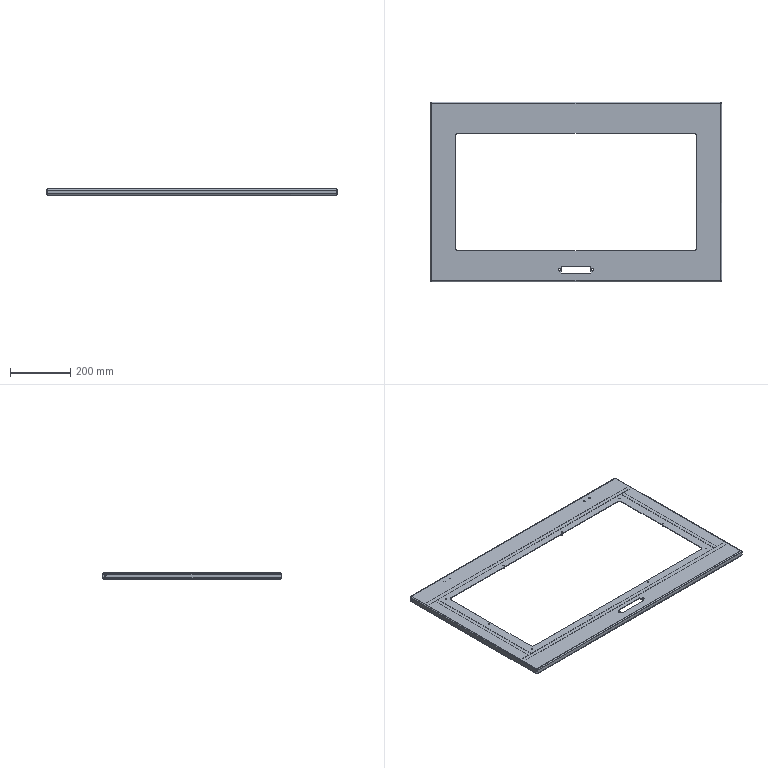Part | NX | features BREP 5 | 5 solids | 264 faces | box 963 x 595 x 20 mm | volume 863102 mm3 | plane 144 | cylinder 76 | cone 28 | spline 16 | commonest cylinder face diameters 5 x20 4 x18 8 x14 6 x8 7 x8 6.5 x4